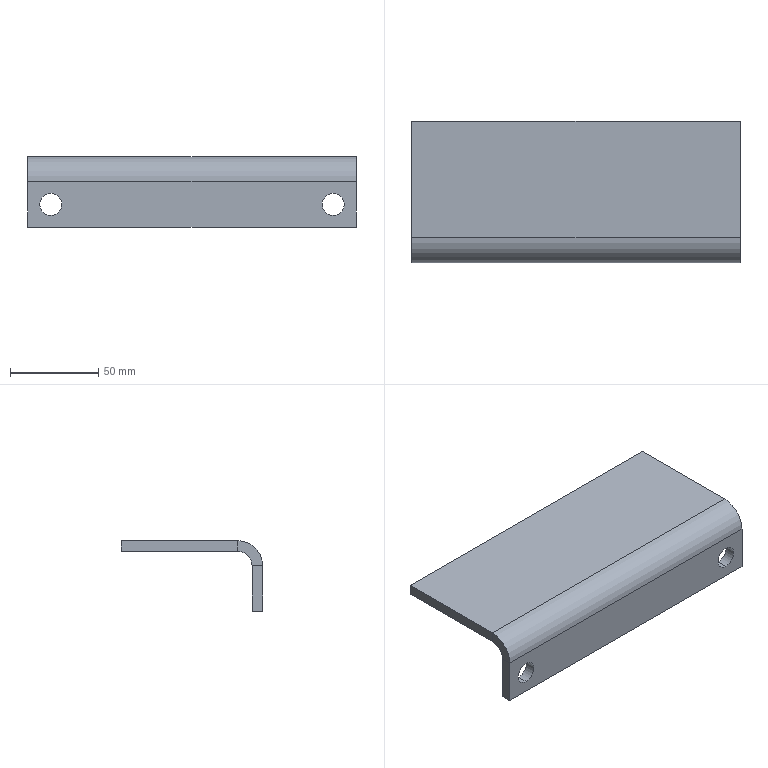Part | SolidWorks | features FlatPattern 1, ICE 1, SMBaseFlange 1, SheetMetal 1 | 1 solid | 18 faces | box 186 x 80 x 40 mm | volume 120482 mm3 | plane 12 | cylinder 6 | commonest cylinder face diameters 12.5 x4 16 x1 28 x1
STEP:
#1=CARTESIAN_POINT('',(13.,0.,6.75));
#2=VERTEX_POINT('',#1);
#3=CARTESIAN_POINT('',(13.,0.,19.25));
#4=VERTEX_POINT('',#3);
#5=CARTESIAN_POINT('',(13.,0.,13.));
#6=DIRECTION('',(0.,1.,0.));
#7=DIRECTION('',(0.,0.,-1.));
#8=AXIS2_PLACEMENT_3D('',#5,#6,#7);
#9=CIRCLE('',#8,6.25);
#10=EDGE_CURVE('',#2,#4,#9,.T.);
#11=ORIENTED_EDGE('',*,*,#10,.F.);
#12=CARTESIAN_POINT('',(13.,6.,6.75));
#13=VERTEX_POINT('',#12);
#14=CARTESIAN_POINT('',(13.,-0.001,6.75));
#15=DIRECTION('',(0.,1.,0.));
#16=VECTOR('',#15,1000.);
#17=LINE('',#14,#16);
#18=EDGE_CURVE('',#2,#13,#17,.T.);
#19=ORIENTED_EDGE('',*,*,#18,.T.);
#20=CARTESIAN_POINT('',(13.,6.,19.25));
#21=VERTEX_POINT('',#20);
#22=CARTESIAN_POINT('',(13.,6.,13.));
#23=DIRECTION('',(0.,1.,0.));
#24=DIRECTION('',(0.,0.,1.));
#25=AXIS2_PLACEMENT_3D('',#22,#23,#24);
#26=CIRCLE('',#25,6.25);
#27=EDGE_CURVE('',#13,#21,#26,.T.);
#28=ORIENTED_EDGE('',*,*,#27,.T.);
#29=CARTESIAN_POINT('',(13.,-0.001,19.25));
#30=DIRECTION('',(0.,1.,0.));
#31=VECTOR('',#30,1000.);
#32=LINE('',#29,#31);
#33=EDGE_CURVE('',#4,#21,#32,.T.);
#34=ORIENTED_EDGE('',*,*,#33,.F.);
#35=EDGE_LOOP('',(#11,#19,#28,#34));
#36=FACE_OUTER_BOUND('',#35,.T.);
#37=CARTESIAN_POINT('',(13.,-0.001,13.));
#38=DIRECTION('',(0.,1.,0.));
#39=DIRECTION('',(0.,0.,1.));
#40=AXIS2_PLACEMENT_3D('',#37,#38,#39);
#41=CYLINDRICAL_SURFACE('',#40,6.25);
#42=ADVANCED_FACE('',(#36),#41,.F.);
#43=CARTESIAN_POINT('',(173.,0.,6.75));
#44=VERTEX_POINT('',#43);
#45=CARTESIAN_POINT('',(173.,0.,19.25));
#46=VERTEX_POINT('',#45);
#47=CARTESIAN_POINT('',(173.,0.,13.));
#48=DIRECTION('',(0.,1.,0.));
#49=DIRECTION('',(0.,0.,-1.));
#50=AXIS2_PLACEMENT_3D('',#47,#48,#49);
#51=CIRCLE('',#50,6.25);
#52=EDGE_CURVE('',#44,#46,#51,.T.);
#53=ORIENTED_EDGE('',*,*,#52,.F.);
#54=CARTESIAN_POINT('',(173.,6.,6.75));
#55=VERTEX_POINT('',#54);
#56=CARTESIAN_POINT('',(173.,-0.001,6.75));
#57=DIRECTION('',(0.,1.,0.));
#58=VECTOR('',#57,1000.);
#59=LINE('',#56,#58);
#60=EDGE_CURVE('',#44,#55,#59,.T.);
#61=ORIENTED_EDGE('',*,*,#60,.T.);
#62=CARTESIAN_POINT('',(173.,6.,19.25));
#63=VERTEX_POINT('',#62);
#64=CARTESIAN_POINT('',(173.,6.,13.));
#65=DIRECTION('',(0.,1.,0.));
#66=DIRECTION('',(0.,0.,1.));
#67=AXIS2_PLACEMENT_3D('',#64,#65,#66);
#68=CIRCLE('',#67,6.25);
#69=EDGE_CURVE('',#55,#63,#68,.T.);
#70=ORIENTED_EDGE('',*,*,#69,.T.);
#71=CARTESIAN_POINT('',(173.,-0.001,19.25));
#72=DIRECTION('',(0.,1.,0.));
#73=VECTOR('',#72,1000.);
#74=LINE('',#71,#73);
#75=EDGE_CURVE('',#46,#63,#74,.T.);
#76=ORIENTED_EDGE('',*,*,#75,.F.);
#77=EDGE_LOOP('',(#53,#61,#70,#76));
#78=FACE_OUTER_BOUND('',#77,.T.);
#79=CARTESIAN_POINT('',(173.,-0.001,13.));
#80=DIRECTION('',(0.,1.,0.));
#81=DIRECTION('',(0.,0.,1.));
#82=AXIS2_PLACEMENT_3D('',#79,#80,#81);
#83=CYLINDRICAL_SURFACE('',#82,6.25);
#84=ADVANCED_FACE('',(#78),#83,.F.);
#85=CARTESIAN_POINT('',(186.,14.,40.));
#86=VERTEX_POINT('',#85);
#87=CARTESIAN_POINT('',(186.,14.,34.));
#88=VERTEX_POINT('',#87);
#89=CARTESIAN_POINT('',(186.,14.,40.));
#90=DIRECTION('',(0.,0.,-1.));
#91=VECTOR('',#90,1000.);
#92=LINE('',#89,#91);
#93=EDGE_CURVE('',#86,#88,#92,.T.);
#94=ORIENTED_EDGE('',*,*,#93,.F.);
#95=CARTESIAN_POINT('',(186.,0.,26.));
#96=VERTEX_POINT('',#95);
#97=CARTESIAN_POINT('',(186.,14.,26.));
#98=DIRECTION('',(-1.,0.,0.));
#99=DIRECTION('',(0.,0.,-1.));
#100=AXIS2_PLACEMENT_3D('',#97,#98,#99);
#101=CIRCLE('',#100,14.);
#102=EDGE_CURVE('',#96,#86,#101,.T.);
#103=ORIENTED_EDGE('',*,*,#102,.F.);
#104=CARTESIAN_POINT('',(186.,6.,26.));
#105=VERTEX_POINT('',#104);
#106=CARTESIAN_POINT('',(186.,6.,26.));
#107=DIRECTION('',(0.,-1.,0.));
#108=VECTOR('',#107,1000.);
#109=LINE('',#106,#108);
#110=EDGE_CURVE('',#105,#96,#109,.T.);
#111=ORIENTED_EDGE('',*,*,#110,.F.);
#112=CARTESIAN_POINT('',(186.,14.,26.));
#113=DIRECTION('',(-1.,0.,0.));
#114=DIRECTION('',(0.,0.,-1.));
#115=AXIS2_PLACEMENT_3D('',#112,#113,#114);
#116=CIRCLE('',#115,8.);
#117=EDGE_CURVE('',#105,#88,#116,.T.);
#118=ORIENTED_EDGE('',*,*,#117,.T.);
#119=EDGE_LOOP('',(#94,#103,#111,#118));
#120=FACE_OUTER_BOUND('',#119,.T.);
#121=CARTESIAN_POINT('',(186.,14.,40.));
#122=DIRECTION('',(1.,0.,0.));
#123=DIRECTION('',(0.,0.,-1.));
#124=AXIS2_PLACEMENT_3D('',#121,#122,#123);
#125=PLANE('',#124);
#126=ADVANCED_FACE('',(#120),#125,.T.);
#127=CARTESIAN_POINT('',(186.,80.,40.));
#128=VERTEX_POINT('',#127);
#129=CARTESIAN_POINT('',(186.,0.,40.));
#130=DIRECTION('',(0.,1.,0.));
#131=VECTOR('',#130,1000.);
#132=LINE('',#129,#131);
#133=EDGE_CURVE('',#86,#128,#132,.T.);
#134=ORIENTED_EDGE('',*,*,#133,.F.);
#135=ORIENTED_EDGE('',*,*,#93,.T.);
#136=CARTESIAN_POINT('',(186.,80.,34.));
#137=VERTEX_POINT('',#136);
#138=CARTESIAN_POINT('',(186.,0.,34.));
#139=DIRECTION('',(0.,1.,0.));
#140=VECTOR('',#139,1000.);
#141=LINE('',#138,#140);
#142=EDGE_CURVE('',#88,#137,#141,.T.);
#143=ORIENTED_EDGE('',*,*,#142,.T.);
#144=CARTESIAN_POINT('',(186.,80.,40.));
#145=DIRECTION('',(0.,0.,-1.));
#146=VECTOR('',#145,1000.);
#147=LINE('',#144,#146);
#148=EDGE_CURVE('',#128,#137,#147,.T.);
#149=ORIENTED_EDGE('',*,*,#148,.F.);
#150=EDGE_LOOP('',(#134,#135,#143,#149));
#151=FACE_OUTER_BOUND('',#150,.T.);
#152=CARTESIAN_POINT('',(186.,6.,26.));
#153=DIRECTION('',(1.,0.,0.));
#154=DIRECTION('',(0.,0.,-1.));
#155=AXIS2_PLACEMENT_3D('',#152,#153,#154);
#156=PLANE('',#155);
#157=ADVANCED_FACE('',(#151),#156,.T.);
#158=CARTESIAN_POINT('',(0.,0.,26.));
#159=VERTEX_POINT('',#158);
#160=CARTESIAN_POINT('',(0.,6.,26.));
#161=VERTEX_POINT('',#160);
#162=CARTESIAN_POINT('',(0.,0.,26.));
#163=DIRECTION('',(0.,1.,0.));
#164=VECTOR('',#163,1000.);
#165=LINE('',#162,#164);
#166=EDGE_CURVE('',#159,#161,#165,.T.);
#167=ORIENTED_EDGE('',*,*,#166,.F.);
#168=CARTESIAN_POINT('',(0.,14.,40.));
#169=VERTEX_POINT('',#168);
#170=CARTESIAN_POINT('',(0.,14.,26.));
#171=DIRECTION('',(-1.,0.,0.));
#172=DIRECTION('',(0.,0.,-1.));
#173=AXIS2_PLACEMENT_3D('',#170,#171,#172);
#174=CIRCLE('',#173,14.);
#175=EDGE_CURVE('',#159,#169,#174,.T.);
#176=ORIENTED_EDGE('',*,*,#175,.T.);
#177=CARTESIAN_POINT('',(0.,14.,34.));
#178=VERTEX_POINT('',#177);
#179=CARTESIAN_POINT('',(0.,14.,34.));
#180=DIRECTION('',(0.,0.,1.));
#181=VECTOR('',#180,1000.);
#182=LINE('',#179,#181);
#183=EDGE_CURVE('',#178,#169,#182,.T.);
#184=ORIENTED_EDGE('',*,*,#183,.F.);
#185=CARTESIAN_POINT('',(0.,14.,26.));
#186=DIRECTION('',(-1.,0.,0.));
#187=DIRECTION('',(0.,0.,-1.));
#188=AXIS2_PLACEMENT_3D('',#185,#186,#187);
#189=CIRCLE('',#188,8.);
#190=EDGE_CURVE('',#161,#178,#189,.T.);
#191=ORIENTED_EDGE('',*,*,#190,.F.);
#192=EDGE_LOOP('',(#167,#176,#184,#191));
#193=FACE_OUTER_BOUND('',#192,.T.);
#194=CARTESIAN_POINT('',(0.,0.,26.));
#195=DIRECTION('',(-1.,0.,0.));
#196=DIRECTION('',(0.,0.,1.));
#197=AXIS2_PLACEMENT_3D('',#194,#195,#196);
#198=PLANE('',#197);
#199=ADVANCED_FACE('',(#193),#198,.T.);
#200=CARTESIAN_POINT('',(0.,0.,0.));
#201=VERTEX_POINT('',#200);
#202=CARTESIAN_POINT('',(0.,0.,0.));
#203=DIRECTION('',(0.,0.,1.));
#204=VECTOR('',#203,1000.);
#205=LINE('',#202,#204);
#206=EDGE_CURVE('',#201,#159,#205,.T.);
#207=ORIENTED_EDGE('',*,*,#206,.T.);
#208=ORIENTED_EDGE('',*,*,#166,.T.);
#209=CARTESIAN_POINT('',(0.,6.,0.));
#210=VERTEX_POINT('',#209);
#211=CARTESIAN_POINT('',(0.,6.,0.));
#212=DIRECTION('',(0.,0.,1.));
#213=VECTOR('',#212,1000.);
#214=LINE('',#211,#213);
#215=EDGE_CURVE('',#210,#161,#214,.T.);
#216=ORIENTED_EDGE('',*,*,#215,.F.);
#217=CARTESIAN_POINT('',(0.,6.,0.));
#218=DIRECTION('',(0.,-1.,0.));
#219=VECTOR('',#218,1000.);
#220=LINE('',#217,#219);
#221=EDGE_CURVE('',#210,#201,#220,.T.);
#222=ORIENTED_EDGE('',*,*,#221,.T.);
#223=EDGE_LOOP('',(#207,#208,#216,#222));
#224=FACE_OUTER_BOUND('',#223,.T.);
#225=CARTESIAN_POINT('',(0.,14.,34.));
#226=DIRECTION('',(-1.,0.,0.));
#227=DIRECTION('',(0.,0.,1.));
#228=AXIS2_PLACEMENT_3D('',#225,#226,#227);
#229=PLANE('',#228);
#230=ADVANCED_FACE('',(#224),#229,.T.);
#231=CARTESIAN_POINT('',(0.,80.,34.));
#232=VERTEX_POINT('',#231);
#233=CARTESIAN_POINT('',(0.,0.,34.));
#234=DIRECTION('',(0.,1.,0.));
#235=VECTOR('',#234,1000.);
#236=LINE('',#233,#235);
#237=EDGE_CURVE('',#178,#232,#236,.T.);
#238=ORIENTED_EDGE('',*,*,#237,.T.);
#239=CARTESIAN_POINT('',(186.,80.,34.));
#240=DIRECTION('',(-1.,0.,0.));
#241=VECTOR('',#240,1000.);
#242=LINE('',#239,#241);
#243=EDGE_CURVE('',#137,#232,#242,.T.);
#244=ORIENTED_EDGE('',*,*,#243,.F.);
#245=ORIENTED_EDGE('',*,*,#142,.F.);
#246=CARTESIAN_POINT('',(186.,14.,34.));
#247=DIRECTION('',(-1.,0.,0.));
#248=VECTOR('',#247,1000.);
#249=LINE('',#246,#248);
#250=EDGE_CURVE('',#88,#178,#249,.T.);
#251=ORIENTED_EDGE('',*,*,#250,.T.);
#252=EDGE_LOOP('',(#238,#244,#245,#251));
#253=FACE_OUTER_BOUND('',#252,.T.);
#254=CARTESIAN_POINT('',(186.,0.,34.));
#255=DIRECTION('',(0.,0.,1.));
#256=DIRECTION('',(1.,0.,0.));
#257=AXIS2_PLACEMENT_3D('',#254,#255,#256);
#258=PLANE('',#257);
#259=ADVANCED_FACE('',(#253),#258,.F.);
#260=CARTESIAN_POINT('',(0.,80.,40.));
#261=VERTEX_POINT('',#260);
#262=CARTESIAN_POINT('',(0.,80.,40.));
#263=DIRECTION('',(0.,0.,-1.));
#264=VECTOR('',#263,1000.);
#265=LINE('',#262,#264);
#266=EDGE_CURVE('',#261,#232,#265,.T.);
#267=ORIENTED_EDGE('',*,*,#266,.F.);
#268=CARTESIAN_POINT('',(186.,80.,40.));
#269=DIRECTION('',(-1.,0.,0.));
#270=VECTOR('',#269,1000.);
#271=LINE('',#268,#270);
#272=EDGE_CURVE('',#128,#261,#271,.T.);
#273=ORIENTED_EDGE('',*,*,#272,.F.);
#274=ORIENTED_EDGE('',*,*,#148,.T.);
#275=ORIENTED_EDGE('',*,*,#243,.T.);
#276=EDGE_LOOP('',(#267,#273,#274,#275));
#277=FACE_OUTER_BOUND('',#276,.T.);
#278=CARTESIAN_POINT('',(186.,80.,40.));
#279=DIRECTION('',(0.,1.,0.));
#280=DIRECTION('',(0.,0.,1.));
#281=AXIS2_PLACEMENT_3D('',#278,#279,#280);
#282=PLANE('',#281);
#283=ADVANCED_FACE('',(#277),#282,.T.);
#284=CARTESIAN_POINT('',(0.,0.,40.));
#285=DIRECTION('',(0.,1.,0.));
#286=VECTOR('',#285,1000.);
#287=LINE('',#284,#286);
#288=EDGE_CURVE('',#169,#261,#287,.T.);
#289=ORIENTED_EDGE('',*,*,#288,.F.);
#290=CARTESIAN_POINT('',(186.,14.,40.));
#291=DIRECTION('',(-1.,0.,0.));
#292=VECTOR('',#291,1000.);
#293=LINE('',#290,#292);
#294=EDGE_CURVE('',#86,#169,#293,.T.);
#295=ORIENTED_EDGE('',*,*,#294,.F.);
#296=ORIENTED_EDGE('',*,*,#133,.T.);
#297=ORIENTED_EDGE('',*,*,#272,.T.);
#298=EDGE_LOOP('',(#289,#295,#296,#297));
#299=FACE_OUTER_BOUND('',#298,.T.);
#300=CARTESIAN_POINT('',(186.,0.,40.));
#301=DIRECTION('',(0.,0.,1.));
#302=DIRECTION('',(1.,0.,0.));
#303=AXIS2_PLACEMENT_3D('',#300,#301,#302);
#304=PLANE('',#303);
#305=ADVANCED_FACE('',(#299),#304,.T.);
#306=ORIENTED_EDGE('',*,*,#175,.F.);
#307=CARTESIAN_POINT('',(186.,0.,26.));
#308=DIRECTION('',(-1.,0.,0.));
#309=VECTOR('',#308,1000.);
#310=LINE('',#307,#309);
#311=EDGE_CURVE('',#96,#159,#310,.T.);
#312=ORIENTED_EDGE('',*,*,#311,.F.);
#313=ORIENTED_EDGE('',*,*,#102,.T.);
#314=ORIENTED_EDGE('',*,*,#294,.T.);
#315=EDGE_LOOP('',(#306,#312,#313,#314));
#316=FACE_OUTER_BOUND('',#315,.T.);
#317=CARTESIAN_POINT('',(186.,14.,26.));
#318=DIRECTION('',(-1.,0.,0.));
#319=DIRECTION('',(0.,0.,1.));
#320=AXIS2_PLACEMENT_3D('',#317,#318,#319);
#321=CYLINDRICAL_SURFACE('',#320,14.);
#322=ADVANCED_FACE('',(#316),#321,.T.);
#323=CARTESIAN_POINT('',(13.,0.,13.));
#324=DIRECTION('',(0.,1.,0.));
#325=DIRECTION('',(0.,0.,-1.));
#326=AXIS2_PLACEMENT_3D('',#323,#324,#325);
#327=CIRCLE('',#326,6.25);
#328=EDGE_CURVE('',#4,#2,#327,.T.);
#329=ORIENTED_EDGE('',*,*,#328,.T.);
#330=ORIENTED_EDGE('',*,*,#10,.T.);
#331=EDGE_LOOP('',(#329,#330));
#332=FACE_BOUND('',#331,.T.);
#333=CARTESIAN_POINT('',(173.,0.,13.));
#334=DIRECTION('',(0.,1.,0.));
#335=DIRECTION('',(0.,0.,-1.));
#336=AXIS2_PLACEMENT_3D('',#333,#334,#335);
#337=CIRCLE('',#336,6.25);
#338=EDGE_CURVE('',#46,#44,#337,.T.);
#339=ORIENTED_EDGE('',*,*,#338,.T.);
#340=ORIENTED_EDGE('',*,*,#52,.T.);
#341=EDGE_LOOP('',(#339,#340));
#342=FACE_BOUND('',#341,.T.);
#343=ORIENTED_EDGE('',*,*,#206,.F.);
#344=CARTESIAN_POINT('',(186.,0.,0.));
#345=VERTEX_POINT('',#344);
#346=CARTESIAN_POINT('',(186.,0.,0.));
#347=DIRECTION('',(-1.,0.,0.));
#348=VECTOR('',#347,1000.);
#349=LINE('',#346,#348);
#350=EDGE_CURVE('',#345,#201,#349,.T.);
#351=ORIENTED_EDGE('',*,*,#350,.F.);
#352=CARTESIAN_POINT('',(186.,0.,0.));
#353=DIRECTION('',(0.,0.,1.));
#354=VECTOR('',#353,1000.);
#355=LINE('',#352,#354);
#356=EDGE_CURVE('',#345,#96,#355,.T.);
#357=ORIENTED_EDGE('',*,*,#356,.T.);
#358=ORIENTED_EDGE('',*,*,#311,.T.);
#359=EDGE_LOOP('',(#343,#351,#357,#358));
#360=FACE_OUTER_BOUND('',#359,.T.);
#361=CARTESIAN_POINT('',(186.,0.,0.));
#362=DIRECTION('',(0.,-1.,0.));
#363=DIRECTION('',(0.,0.,-1.));
#364=AXIS2_PLACEMENT_3D('',#361,#362,#363);
#365=PLANE('',#364);
#366=ADVANCED_FACE('',(#332,#342,#360),#365,.T.);
#367=ORIENTED_EDGE('',*,*,#221,.F.);
#368=CARTESIAN_POINT('',(186.,6.,0.));
#369=VERTEX_POINT('',#368);
#370=CARTESIAN_POINT('',(186.,6.,0.));
#371=DIRECTION('',(-1.,0.,0.));
#372=VECTOR('',#371,1000.);
#373=LINE('',#370,#372);
#374=EDGE_CURVE('',#369,#210,#373,.T.);
#375=ORIENTED_EDGE('',*,*,#374,.F.);
#376=CARTESIAN_POINT('',(186.,6.,0.));
#377=DIRECTION('',(0.,-1.,0.));
#378=VECTOR('',#377,1000.);
#379=LINE('',#376,#378);
#380=EDGE_CURVE('',#369,#345,#379,.T.);
#381=ORIENTED_EDGE('',*,*,#380,.T.);
#382=ORIENTED_EDGE('',*,*,#350,.T.);
#383=EDGE_LOOP('',(#367,#375,#381,#382));
#384=FACE_OUTER_BOUND('',#383,.T.);
#385=CARTESIAN_POINT('',(186.,6.,0.));
#386=DIRECTION('',(0.,0.,-1.));
#387=DIRECTION('',(0.,1.,0.));
#388=AXIS2_PLACEMENT_3D('',#385,#386,#387);
#389=PLANE('',#388);
#390=ADVANCED_FACE('',(#384),#389,.T.);
#391=CARTESIAN_POINT('',(13.,6.,13.));
#392=DIRECTION('',(0.,1.,0.));
#393=DIRECTION('',(0.,0.,1.));
#394=AXIS2_PLACEMENT_3D('',#391,#392,#393);
#395=CIRCLE('',#394,6.25);
#396=EDGE_CURVE('',#21,#13,#395,.T.);
#397=ORIENTED_EDGE('',*,*,#396,.F.);
#398=ORIENTED_EDGE('',*,*,#27,.F.);
#399=EDGE_LOOP('',(#397,#398));
#400=FACE_BOUND('',#399,.T.);
#401=CARTESIAN_POINT('',(173.,6.,13.));
#402=DIRECTION('',(0.,1.,0.));
#403=DIRECTION('',(0.,0.,1.));
#404=AXIS2_PLACEMENT_3D('',#401,#402,#403);
#405=CIRCLE('',#404,6.25);
#406=EDGE_CURVE('',#63,#55,#405,.T.);
#407=ORIENTED_EDGE('',*,*,#406,.F.);
#408=ORIENTED_EDGE('',*,*,#69,.F.);
#409=EDGE_LOOP('',(#407,#408));
#410=FACE_BOUND('',#409,.T.);
#411=ORIENTED_EDGE('',*,*,#215,.T.);
#412=CARTESIAN_POINT('',(186.,6.,26.));
#413=DIRECTION('',(-1.,0.,0.));
#414=VECTOR('',#413,1000.);
#415=LINE('',#412,#414);
#416=EDGE_CURVE('',#105,#161,#415,.T.);
#417=ORIENTED_EDGE('',*,*,#416,.F.);
#418=CARTESIAN_POINT('',(186.,6.,0.));
#419=DIRECTION('',(0.,0.,1.));
#420=VECTOR('',#419,1000.);
#421=LINE('',#418,#420);
#422=EDGE_CURVE('',#369,#105,#421,.T.);
#423=ORIENTED_EDGE('',*,*,#422,.F.);
#424=ORIENTED_EDGE('',*,*,#374,.T.);
#425=EDGE_LOOP('',(#411,#417,#423,#424));
#426=FACE_OUTER_BOUND('',#425,.T.);
#427=CARTESIAN_POINT('',(186.,6.,0.));
#428=DIRECTION('',(0.,-1.,0.));
#429=DIRECTION('',(0.,0.,-1.));
#430=AXIS2_PLACEMENT_3D('',#427,#428,#429);
#431=PLANE('',#430);
#432=ADVANCED_FACE('',(#400,#410,#426),#431,.F.);
#433=ORIENTED_EDGE('',*,*,#190,.T.);
#434=ORIENTED_EDGE('',*,*,#250,.F.);
#435=ORIENTED_EDGE('',*,*,#117,.F.);
#436=ORIENTED_EDGE('',*,*,#416,.T.);
#437=EDGE_LOOP('',(#433,#434,#435,#436));
#438=FACE_OUTER_BOUND('',#437,.T.);
#439=CARTESIAN_POINT('',(186.,14.,26.));
#440=DIRECTION('',(-1.,0.,0.));
#441=DIRECTION('',(0.,0.,1.));
#442=AXIS2_PLACEMENT_3D('',#439,#440,#441);
#443=CYLINDRICAL_SURFACE('',#442,8.);
#444=ADVANCED_FACE('',(#438),#443,.F.);
#445=ORIENTED_EDGE('',*,*,#422,.T.);
#446=ORIENTED_EDGE('',*,*,#110,.T.);
#447=ORIENTED_EDGE('',*,*,#356,.F.);
#448=ORIENTED_EDGE('',*,*,#380,.F.);
#449=EDGE_LOOP('',(#445,#446,#447,#448));
#450=FACE_OUTER_BOUND('',#449,.T.);
#451=CARTESIAN_POINT('',(186.,14.,26.));
#452=DIRECTION('',(1.,0.,0.));
#453=DIRECTION('',(0.,0.,-1.));
#454=AXIS2_PLACEMENT_3D('',#451,#452,#453);
#455=PLANE('',#454);
#456=ADVANCED_FACE('',(#450),#455,.T.);
#457=ORIENTED_EDGE('',*,*,#237,.F.);
#458=ORIENTED_EDGE('',*,*,#183,.T.);
#459=ORIENTED_EDGE('',*,*,#288,.T.);
#460=ORIENTED_EDGE('',*,*,#266,.T.);
#461=EDGE_LOOP('',(#457,#458,#459,#460));
#462=FACE_OUTER_BOUND('',#461,.T.);
#463=CARTESIAN_POINT('',(0.,14.,26.));
#464=DIRECTION('',(1.,0.,0.));
#465=DIRECTION('',(0.,0.,-1.));
#466=AXIS2_PLACEMENT_3D('',#463,#464,#465);
#467=PLANE('',#466);
#468=ADVANCED_FACE('',(#462),#467,.F.);
#469=ORIENTED_EDGE('',*,*,#60,.F.);
#470=ORIENTED_EDGE('',*,*,#338,.F.);
#471=ORIENTED_EDGE('',*,*,#75,.T.);
#472=ORIENTED_EDGE('',*,*,#406,.T.);
#473=EDGE_LOOP('',(#469,#470,#471,#472));
#474=FACE_OUTER_BOUND('',#473,.T.);
#475=CARTESIAN_POINT('',(173.,-0.001,13.));
#476=DIRECTION('',(0.,1.,0.));
#477=DIRECTION('',(0.,0.,1.));
#478=AXIS2_PLACEMENT_3D('',#475,#476,#477);
#479=CYLINDRICAL_SURFACE('',#478,6.25);
#480=ADVANCED_FACE('',(#474),#479,.F.);
#481=ORIENTED_EDGE('',*,*,#18,.F.);
#482=ORIENTED_EDGE('',*,*,#328,.F.);
#483=ORIENTED_EDGE('',*,*,#33,.T.);
#484=ORIENTED_EDGE('',*,*,#396,.T.);
#485=EDGE_LOOP('',(#481,#482,#483,#484));
#486=FACE_OUTER_BOUND('',#485,.T.);
#487=CARTESIAN_POINT('',(13.,-0.001,13.));
#488=DIRECTION('',(0.,1.,0.));
#489=DIRECTION('',(0.,0.,1.));
#490=AXIS2_PLACEMENT_3D('',#487,#488,#489);
#491=CYLINDRICAL_SURFACE('',#490,6.25);
#492=ADVANCED_FACE('',(#486),#491,.F.);
#493=CLOSED_SHELL('',(#42,#84,#126,#157,#199,#230,#259,#283,#305,#322,#366,#390,#432,#444,#456,#468,#480,#492));
#494=MANIFOLD_SOLID_BREP('',#493);
#495=CARTESIAN_POINT('',(0.,0.,0.));
#496=DIRECTION('',(0.,0.,1.));
#497=DIRECTION('',(1.,0.,0.));
#498=AXIS2_PLACEMENT_3D('',#495,#496,#497);
#499=(LENGTH_UNIT()NAMED_UNIT(*)SI_UNIT(.MILLI.,.METRE.));
#500=UNCERTAINTY_MEASURE_WITH_UNIT(LENGTH_MEASURE(0.00001),#499,'','');
#501=(NAMED_UNIT(*)PLANE_ANGLE_UNIT()SI_UNIT($,.RADIAN.));
#502=(NAMED_UNIT(*)SI_UNIT($,.STERADIAN.)SOLID_ANGLE_UNIT());
#503=(GEOMETRIC_REPRESENTATION_CONTEXT(3)GLOBAL_UNCERTAINTY_ASSIGNED_CONTEXT((#500))GLOBAL_UNIT_ASSIGNED_CONTEXT((#499,#501,#502))REPRESENTATION_CONTEXT('',''));
#504=ADVANCED_BREP_SHAPE_REPRESENTATION('',(#494,#498),#503);